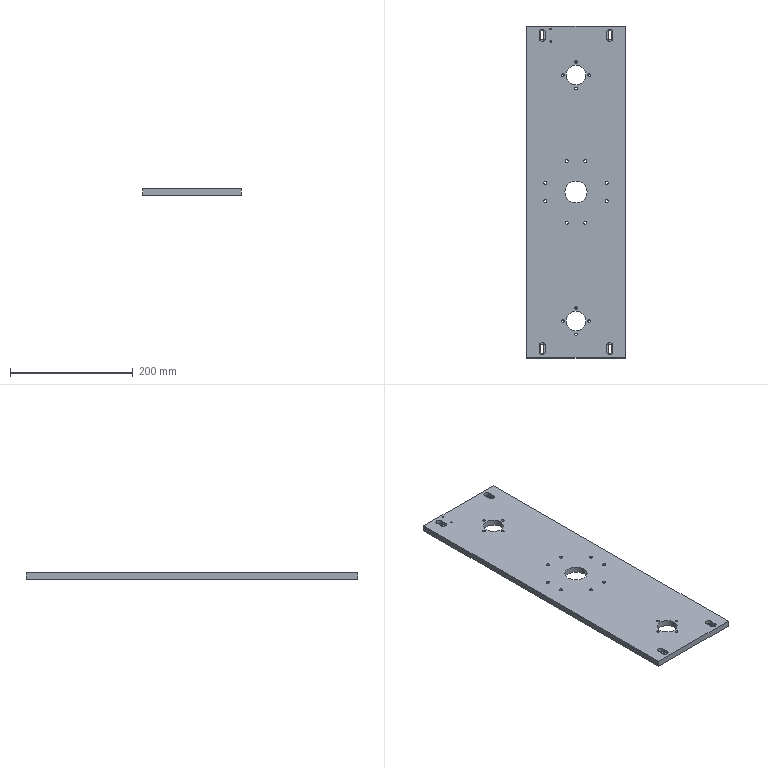Part | SolidWorks | features HoleWzd 7, ICE 4, Extrusion 1 | 1 solid | 84 faces | box 160 x 540 x 10 mm | volume 829534 mm3 | cylinder 58 | plane 26 | commonest cylinder face diameters 4.2 x16 5 x16 5.5 x8 10 x8 2.5 x4 32 x4